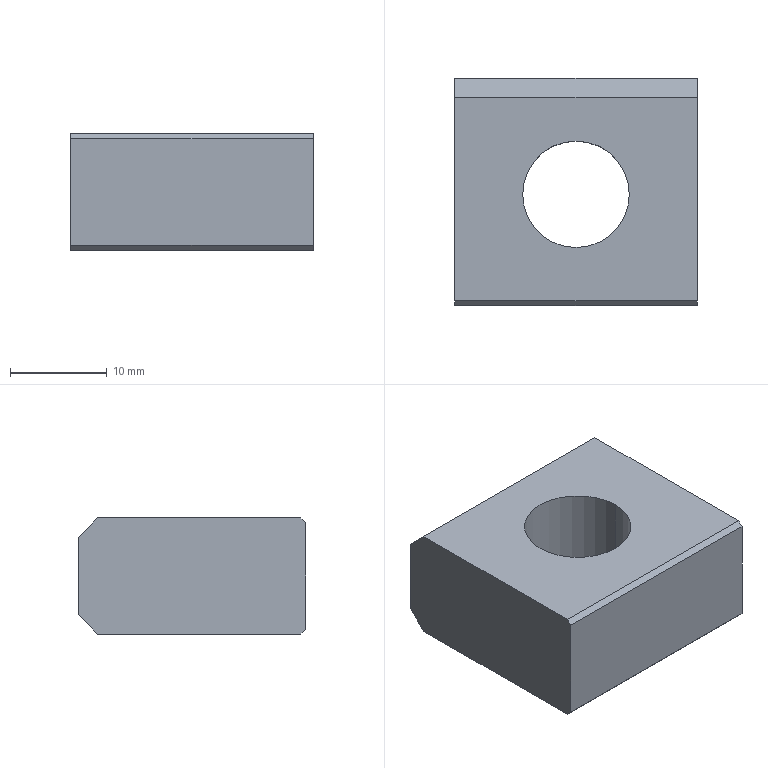Part | STEP file | 1 solid | 12 faces | box 25 x 23.5 x 12 mm | volume 5803 mm3 | plane 10 | cylinder 2 | commonest cylinder face diameters 11 x2
STEP:
#1=CARTESIAN_POINT('',(0.,0.,0.));
#2=DIRECTION('',(0.,0.,1.));
#3=DIRECTION('',(1.,0.,0.));
#4=AXIS2_PLACEMENT_3D('',#1,#2,#3);
#5=CARTESIAN_POINT('',(5.5,-0.25,-12.));
#6=VERTEX_POINT('',#5);
#7=CARTESIAN_POINT('',(5.5,-0.25,0.));
#8=VERTEX_POINT('',#7);
#9=CARTESIAN_POINT('',(5.5,-0.25,-12.));
#10=DIRECTION('',(0.,0.,1.));
#11=VECTOR('',#10,1.);
#12=LINE('',#9,#11);
#13=CARTESIAN_POINT('',(0.,-0.25,-12.));
#14=DIRECTION('',(0.,0.,1.));
#15=DIRECTION('',(1.,0.,0.));
#16=AXIS2_PLACEMENT_3D('',#13,#14,#15);
#17=CYLINDRICAL_SURFACE('',#16,5.5);
#18=CARTESIAN_POINT('',(6.283,0.));
#19=DIRECTION('',(0.,1.));
#20=VECTOR('',#19,1.);
#21=LINE('',#18,#20);
#22=(GEOMETRIC_REPRESENTATION_CONTEXT(2)PARAMETRIC_REPRESENTATION_CONTEXT()REPRESENTATION_CONTEXT('',''));
#23=DEFINITIONAL_REPRESENTATION('',(#21),#22);
#24=PCURVE('',#17,#23);
#25=CARTESIAN_POINT('',(0.,-0.25,-12.));
#26=DIRECTION('',(0.,0.,1.));
#27=DIRECTION('',(1.,0.,0.));
#28=AXIS2_PLACEMENT_3D('',#25,#26,#27);
#29=CYLINDRICAL_SURFACE('',#28,5.5);
#30=CARTESIAN_POINT('',(0.,0.));
#31=DIRECTION('',(0.,1.));
#32=VECTOR('',#31,1.);
#33=LINE('',#30,#32);
#34=(GEOMETRIC_REPRESENTATION_CONTEXT(2)PARAMETRIC_REPRESENTATION_CONTEXT()REPRESENTATION_CONTEXT('',''));
#35=DEFINITIONAL_REPRESENTATION('',(#33),#34);
#36=PCURVE('',#29,#35);
#37=SURFACE_CURVE('',#12,(#24,#36),.PCURVE_S1.);
#38=EDGE_CURVE('',#6,#8,#37,.T.);
#39=ORIENTED_EDGE('',*,*,#38,.T.);
#40=CARTESIAN_POINT('',(-5.5,-0.25,0.));
#41=VERTEX_POINT('',#40);
#42=CARTESIAN_POINT('',(0.,-0.25,0.));
#43=DIRECTION('',(0.,0.,1.));
#44=DIRECTION('',(1.,0.,0.));
#45=AXIS2_PLACEMENT_3D('',#42,#43,#44);
#46=CIRCLE('',#45,5.5);
#47=CARTESIAN_POINT('',(0.,12.));
#48=DIRECTION('',(1.,0.));
#49=VECTOR('',#48,1.);
#50=LINE('',#47,#49);
#51=(GEOMETRIC_REPRESENTATION_CONTEXT(2)PARAMETRIC_REPRESENTATION_CONTEXT()REPRESENTATION_CONTEXT('',''));
#52=DEFINITIONAL_REPRESENTATION('',(#50),#51);
#53=PCURVE('',#17,#52);
#54=CARTESIAN_POINT('',(-12.5,-11.75,0.));
#55=DIRECTION('',(0.,0.,-1.));
#56=DIRECTION('',(-1.,0.,0.));
#57=AXIS2_PLACEMENT_3D('',#54,#55,#56);
#58=PLANE('',#57);
#59=CARTESIAN_POINT('',(-18.,11.5));
#60=CARTESIAN_POINT('',(-18.,21.026));
#61=CARTESIAN_POINT('',(-9.75,16.263));
#62=CARTESIAN_POINT('',(-1.5,11.5));
#63=CARTESIAN_POINT('',(-9.75,6.737));
#64=CARTESIAN_POINT('',(-18.,1.974));
#65=CARTESIAN_POINT('',(-18.,11.5));
#66=(BOUNDED_CURVE()B_SPLINE_CURVE(2,(#59,#60,#61,#62,#63,#64,#65),.UNSPECIFIED.,.T.,.F.)B_SPLINE_CURVE_WITH_KNOTS((1,2,2,2,2,1),(-2.094,0.,2.094,4.189,6.283,8.378),.UNSPECIFIED.)CURVE()GEOMETRIC_REPRESENTATION_ITEM()RATIONAL_B_SPLINE_CURVE((1.,0.5,1.,0.5,1.,0.5,1.))REPRESENTATION_ITEM(''));
#67=(GEOMETRIC_REPRESENTATION_CONTEXT(2)PARAMETRIC_REPRESENTATION_CONTEXT()REPRESENTATION_CONTEXT('',''));
#68=DEFINITIONAL_REPRESENTATION('',(#66),#67);
#69=PCURVE('',#58,#68);
#70=SURFACE_CURVE('',#46,(#53,#69),.PCURVE_S1.);
#71=EDGE_CURVE('',#41,#8,#70,.T.);
#72=ORIENTED_EDGE('',*,*,#71,.F.);
#73=CARTESIAN_POINT('',(-5.5,-0.25,-12.));
#74=VERTEX_POINT('',#73);
#75=CARTESIAN_POINT('',(-5.5,-0.25,-12.));
#76=DIRECTION('',(0.,0.,1.));
#77=VECTOR('',#76,1.);
#78=LINE('',#75,#77);
#79=CARTESIAN_POINT('',(3.142,0.));
#80=DIRECTION('',(0.,1.));
#81=VECTOR('',#80,1.);
#82=LINE('',#79,#81);
#83=(GEOMETRIC_REPRESENTATION_CONTEXT(2)PARAMETRIC_REPRESENTATION_CONTEXT()REPRESENTATION_CONTEXT('',''));
#84=DEFINITIONAL_REPRESENTATION('',(#82),#83);
#85=PCURVE('',#17,#84);
#86=CARTESIAN_POINT('',(3.142,0.));
#87=DIRECTION('',(0.,1.));
#88=VECTOR('',#87,1.);
#89=LINE('',#86,#88);
#90=(GEOMETRIC_REPRESENTATION_CONTEXT(2)PARAMETRIC_REPRESENTATION_CONTEXT()REPRESENTATION_CONTEXT('',''));
#91=DEFINITIONAL_REPRESENTATION('',(#89),#90);
#92=PCURVE('',#29,#91);
#93=SURFACE_CURVE('',#78,(#85,#92),.PCURVE_S1.);
#94=EDGE_CURVE('',#74,#41,#93,.T.);
#95=ORIENTED_EDGE('',*,*,#94,.F.);
#96=CARTESIAN_POINT('',(0.,-0.25,-12.));
#97=DIRECTION('',(0.,0.,1.));
#98=DIRECTION('',(1.,0.,0.));
#99=AXIS2_PLACEMENT_3D('',#96,#97,#98);
#100=CIRCLE('',#99,5.5);
#101=CARTESIAN_POINT('',(0.,0.));
#102=DIRECTION('',(1.,0.));
#103=VECTOR('',#102,1.);
#104=LINE('',#101,#103);
#105=(GEOMETRIC_REPRESENTATION_CONTEXT(2)PARAMETRIC_REPRESENTATION_CONTEXT()REPRESENTATION_CONTEXT('',''));
#106=DEFINITIONAL_REPRESENTATION('',(#104),#105);
#107=PCURVE('',#17,#106);
#108=CARTESIAN_POINT('',(-12.5,-11.75,-12.));
#109=DIRECTION('',(0.,0.,-1.));
#110=DIRECTION('',(-1.,0.,0.));
#111=AXIS2_PLACEMENT_3D('',#108,#109,#110);
#112=PLANE('',#111);
#113=CARTESIAN_POINT('',(-18.,11.5));
#114=CARTESIAN_POINT('',(-18.,21.026));
#115=CARTESIAN_POINT('',(-9.75,16.263));
#116=CARTESIAN_POINT('',(-1.5,11.5));
#117=CARTESIAN_POINT('',(-9.75,6.737));
#118=CARTESIAN_POINT('',(-18.,1.974));
#119=CARTESIAN_POINT('',(-18.,11.5));
#120=(BOUNDED_CURVE()B_SPLINE_CURVE(2,(#113,#114,#115,#116,#117,#118,#119),.UNSPECIFIED.,.T.,.F.)B_SPLINE_CURVE_WITH_KNOTS((1,2,2,2,2,1),(-2.094,0.,2.094,4.189,6.283,8.378),.UNSPECIFIED.)CURVE()GEOMETRIC_REPRESENTATION_ITEM()RATIONAL_B_SPLINE_CURVE((1.,0.5,1.,0.5,1.,0.5,1.))REPRESENTATION_ITEM(''));
#121=(GEOMETRIC_REPRESENTATION_CONTEXT(2)PARAMETRIC_REPRESENTATION_CONTEXT()REPRESENTATION_CONTEXT('',''));
#122=DEFINITIONAL_REPRESENTATION('',(#120),#121);
#123=PCURVE('',#112,#122);
#124=SURFACE_CURVE('',#100,(#107,#123),.PCURVE_S1.);
#125=EDGE_CURVE('',#74,#6,#124,.T.);
#126=ORIENTED_EDGE('',*,*,#125,.T.);
#127=EDGE_LOOP('',(#39,#72,#95,#126));
#128=FACE_BOUND('',#127,.F.);
#129=ADVANCED_FACE('',(#128),#17,.F.);
#130=CARTESIAN_POINT('',(-12.5,9.75,-12.));
#131=VERTEX_POINT('',#130);
#132=CARTESIAN_POINT('',(-12.5,-11.25,-12.));
#133=VERTEX_POINT('',#132);
#134=CARTESIAN_POINT('',(-12.5,11.75,-12.));
#135=DIRECTION('',(0.,-1.,0.));
#136=VECTOR('',#135,1.);
#137=LINE('',#134,#136);
#138=CARTESIAN_POINT('',(-12.5,11.75,-12.));
#139=DIRECTION('',(-1.,0.,0.));
#140=DIRECTION('',(0.,-1.,0.));
#141=AXIS2_PLACEMENT_3D('',#138,#139,#140);
#142=PLANE('',#141);
#143=CARTESIAN_POINT('',(0.,0.));
#144=DIRECTION('',(1.,0.));
#145=VECTOR('',#144,1.);
#146=LINE('',#143,#145);
#147=(GEOMETRIC_REPRESENTATION_CONTEXT(2)PARAMETRIC_REPRESENTATION_CONTEXT()REPRESENTATION_CONTEXT('',''));
#148=DEFINITIONAL_REPRESENTATION('',(#146),#147);
#149=PCURVE('',#142,#148);
#150=CARTESIAN_POINT('',(0.,23.5));
#151=DIRECTION('',(0.,-1.));
#152=VECTOR('',#151,1.);
#153=LINE('',#150,#152);
#154=(GEOMETRIC_REPRESENTATION_CONTEXT(2)PARAMETRIC_REPRESENTATION_CONTEXT()REPRESENTATION_CONTEXT('',''));
#155=DEFINITIONAL_REPRESENTATION('',(#153),#154);
#156=PCURVE('',#112,#155);
#157=SURFACE_CURVE('',#137,(#149,#156),.PCURVE_S1.);
#158=EDGE_CURVE('',#131,#133,#157,.T.);
#159=ORIENTED_EDGE('',*,*,#158,.T.);
#160=CARTESIAN_POINT('',(-12.5,-11.75,-11.5));
#161=VERTEX_POINT('',#160);
#162=CARTESIAN_POINT('',(-12.5,0.25,-23.5));
#163=DIRECTION('',(0.,-0.7071,0.7071));
#164=VECTOR('',#163,1.);
#165=LINE('',#162,#164);
#166=CARTESIAN_POINT('',(11.5,-11.5));
#167=DIRECTION('',(0.7071,0.7071));
#168=VECTOR('',#167,1.);
#169=LINE('',#166,#168);
#170=(GEOMETRIC_REPRESENTATION_CONTEXT(2)PARAMETRIC_REPRESENTATION_CONTEXT()REPRESENTATION_CONTEXT('',''));
#171=DEFINITIONAL_REPRESENTATION('',(#169),#170);
#172=PCURVE('',#142,#171);
#173=CARTESIAN_POINT('',(12.5,-11.75,-11.5));
#174=DIRECTION('',(0.,0.7071,0.7071));
#175=DIRECTION('',(0.,-0.7071,0.7071));
#176=AXIS2_PLACEMENT_3D('',#173,#174,#175);
#177=PLANE('',#176);
#178=CARTESIAN_POINT('',(-16.971,-25.));
#179=DIRECTION('',(1.,0.));
#180=VECTOR('',#179,1.);
#181=LINE('',#178,#180);
#182=(GEOMETRIC_REPRESENTATION_CONTEXT(2)PARAMETRIC_REPRESENTATION_CONTEXT()REPRESENTATION_CONTEXT('',''));
#183=DEFINITIONAL_REPRESENTATION('',(#181),#182);
#184=PCURVE('',#177,#183);
#185=SURFACE_CURVE('',#165,(#172,#184),.PCURVE_S1.);
#186=EDGE_CURVE('',#133,#161,#185,.T.);
#187=ORIENTED_EDGE('',*,*,#186,.T.);
#188=CARTESIAN_POINT('',(-12.5,-11.75,-0.5));
#189=VERTEX_POINT('',#188);
#190=CARTESIAN_POINT('',(-12.5,-11.75,-12.));
#191=DIRECTION('',(0.,0.,1.));
#192=VECTOR('',#191,1.);
#193=LINE('',#190,#192);
#194=CARTESIAN_POINT('',(23.5,0.));
#195=DIRECTION('',(0.,1.));
#196=VECTOR('',#195,1.);
#197=LINE('',#194,#196);
#198=(GEOMETRIC_REPRESENTATION_CONTEXT(2)PARAMETRIC_REPRESENTATION_CONTEXT()REPRESENTATION_CONTEXT('',''));
#199=DEFINITIONAL_REPRESENTATION('',(#197),#198);
#200=PCURVE('',#142,#199);
#201=CARTESIAN_POINT('',(12.5,-11.75,-12.));
#202=DIRECTION('',(0.,-1.,0.));
#203=DIRECTION('',(1.,0.,0.));
#204=AXIS2_PLACEMENT_3D('',#201,#202,#203);
#205=PLANE('',#204);
#206=CARTESIAN_POINT('',(-25.,0.));
#207=DIRECTION('',(0.,1.));
#208=VECTOR('',#207,1.);
#209=LINE('',#206,#208);
#210=(GEOMETRIC_REPRESENTATION_CONTEXT(2)PARAMETRIC_REPRESENTATION_CONTEXT()REPRESENTATION_CONTEXT('',''));
#211=DEFINITIONAL_REPRESENTATION('',(#209),#210);
#212=PCURVE('',#205,#211);
#213=SURFACE_CURVE('',#193,(#200,#212),.PCURVE_S1.);
#214=EDGE_CURVE('',#161,#189,#213,.T.);
#215=ORIENTED_EDGE('',*,*,#214,.T.);
#216=CARTESIAN_POINT('',(-12.5,-11.25,0.));
#217=VERTEX_POINT('',#216);
#218=CARTESIAN_POINT('',(-12.5,-5.75,5.5));
#219=DIRECTION('',(0.,0.7071,0.7071));
#220=VECTOR('',#219,1.);
#221=LINE('',#218,#220);
#222=CARTESIAN_POINT('',(17.5,17.5));
#223=DIRECTION('',(-0.7071,0.7071));
#224=VECTOR('',#223,1.);
#225=LINE('',#222,#224);
#226=(GEOMETRIC_REPRESENTATION_CONTEXT(2)PARAMETRIC_REPRESENTATION_CONTEXT()REPRESENTATION_CONTEXT('',''));
#227=DEFINITIONAL_REPRESENTATION('',(#225),#226);
#228=PCURVE('',#142,#227);
#229=CARTESIAN_POINT('',(-12.5,-11.25,0.));
#230=DIRECTION('',(0.,-0.7071,0.7071));
#231=DIRECTION('',(0.,-0.7071,-0.7071));
#232=AXIS2_PLACEMENT_3D('',#229,#230,#231);
#233=PLANE('',#232);
#234=CARTESIAN_POINT('',(-7.778,0.));
#235=DIRECTION('',(-1.,0.));
#236=VECTOR('',#235,1.);
#237=LINE('',#234,#236);
#238=(GEOMETRIC_REPRESENTATION_CONTEXT(2)PARAMETRIC_REPRESENTATION_CONTEXT()REPRESENTATION_CONTEXT('',''));
#239=DEFINITIONAL_REPRESENTATION('',(#237),#238);
#240=PCURVE('',#233,#239);
#241=SURFACE_CURVE('',#221,(#228,#240),.PCURVE_S1.);
#242=EDGE_CURVE('',#189,#217,#241,.T.);
#243=ORIENTED_EDGE('',*,*,#242,.T.);
#244=CARTESIAN_POINT('',(-12.5,9.75,0.));
#245=VERTEX_POINT('',#244);
#246=CARTESIAN_POINT('',(-12.5,11.75,0.));
#247=DIRECTION('',(0.,-1.,0.));
#248=VECTOR('',#247,1.);
#249=LINE('',#246,#248);
#250=CARTESIAN_POINT('',(0.,12.));
#251=DIRECTION('',(1.,0.));
#252=VECTOR('',#251,1.);
#253=LINE('',#250,#252);
#254=(GEOMETRIC_REPRESENTATION_CONTEXT(2)PARAMETRIC_REPRESENTATION_CONTEXT()REPRESENTATION_CONTEXT('',''));
#255=DEFINITIONAL_REPRESENTATION('',(#253),#254);
#256=PCURVE('',#142,#255);
#257=CARTESIAN_POINT('',(0.,23.5));
#258=DIRECTION('',(0.,-1.));
#259=VECTOR('',#258,1.);
#260=LINE('',#257,#259);
#261=(GEOMETRIC_REPRESENTATION_CONTEXT(2)PARAMETRIC_REPRESENTATION_CONTEXT()REPRESENTATION_CONTEXT('',''));
#262=DEFINITIONAL_REPRESENTATION('',(#260),#261);
#263=PCURVE('',#58,#262);
#264=SURFACE_CURVE('',#249,(#256,#263),.PCURVE_S1.);
#265=EDGE_CURVE('',#245,#217,#264,.T.);
#266=ORIENTED_EDGE('',*,*,#265,.F.);
#267=CARTESIAN_POINT('',(-12.5,11.75,-2.));
#268=VERTEX_POINT('',#267);
#269=CARTESIAN_POINT('',(-12.5,16.75,-7.));
#270=DIRECTION('',(0.,0.7071,-0.7071));
#271=VECTOR('',#270,1.);
#272=LINE('',#269,#271);
#273=CARTESIAN_POINT('',(-5.,5.));
#274=DIRECTION('',(-0.7071,-0.7071));
#275=VECTOR('',#274,1.);
#276=LINE('',#273,#275);
#277=(GEOMETRIC_REPRESENTATION_CONTEXT(2)PARAMETRIC_REPRESENTATION_CONTEXT()REPRESENTATION_CONTEXT('',''));
#278=DEFINITIONAL_REPRESENTATION('',(#276),#277);
#279=PCURVE('',#142,#278);
#280=CARTESIAN_POINT('',(-12.5,9.75,0.));
#281=DIRECTION('',(0.,0.7071,0.7071));
#282=DIRECTION('',(0.,-0.7071,0.7071));
#283=AXIS2_PLACEMENT_3D('',#280,#281,#282);
#284=PLANE('',#283);
#285=CARTESIAN_POINT('',(-9.899,0.));
#286=DIRECTION('',(-1.,0.));
#287=VECTOR('',#286,1.);
#288=LINE('',#285,#287);
#289=(GEOMETRIC_REPRESENTATION_CONTEXT(2)PARAMETRIC_REPRESENTATION_CONTEXT()REPRESENTATION_CONTEXT('',''));
#290=DEFINITIONAL_REPRESENTATION('',(#288),#289);
#291=PCURVE('',#284,#290);
#292=SURFACE_CURVE('',#272,(#279,#291),.PCURVE_S1.);
#293=EDGE_CURVE('',#245,#268,#292,.T.);
#294=ORIENTED_EDGE('',*,*,#293,.T.);
#295=CARTESIAN_POINT('',(-12.5,11.75,-10.));
#296=VERTEX_POINT('',#295);
#297=CARTESIAN_POINT('',(-12.5,11.75,-12.));
#298=DIRECTION('',(0.,0.,1.));
#299=VECTOR('',#298,1.);
#300=LINE('',#297,#299);
#301=CARTESIAN_POINT('',(0.,0.));
#302=DIRECTION('',(0.,1.));
#303=VECTOR('',#302,1.);
#304=LINE('',#301,#303);
#305=(GEOMETRIC_REPRESENTATION_CONTEXT(2)PARAMETRIC_REPRESENTATION_CONTEXT()REPRESENTATION_CONTEXT('',''));
#306=DEFINITIONAL_REPRESENTATION('',(#304),#305);
#307=PCURVE('',#142,#306);
#308=CARTESIAN_POINT('',(12.5,11.75,-12.));
#309=DIRECTION('',(0.,1.,0.));
#310=DIRECTION('',(-1.,0.,0.));
#311=AXIS2_PLACEMENT_3D('',#308,#309,#310);
#312=PLANE('',#311);
#313=CARTESIAN_POINT('',(25.,0.));
#314=DIRECTION('',(0.,1.));
#315=VECTOR('',#314,1.);
#316=LINE('',#313,#315);
#317=(GEOMETRIC_REPRESENTATION_CONTEXT(2)PARAMETRIC_REPRESENTATION_CONTEXT()REPRESENTATION_CONTEXT('',''));
#318=DEFINITIONAL_REPRESENTATION('',(#316),#317);
#319=PCURVE('',#312,#318);
#320=SURFACE_CURVE('',#300,(#307,#319),.PCURVE_S1.);
#321=EDGE_CURVE('',#296,#268,#320,.T.);
#322=ORIENTED_EDGE('',*,*,#321,.F.);
#323=CARTESIAN_POINT('',(-12.5,10.75,-11.));
#324=DIRECTION('',(0.,-0.7071,-0.7071));
#325=VECTOR('',#324,1.);
#326=LINE('',#323,#325);
#327=CARTESIAN_POINT('',(1.,1.));
#328=DIRECTION('',(0.7071,-0.7071));
#329=VECTOR('',#328,1.);
#330=LINE('',#327,#329);
#331=(GEOMETRIC_REPRESENTATION_CONTEXT(2)PARAMETRIC_REPRESENTATION_CONTEXT()REPRESENTATION_CONTEXT('',''));
#332=DEFINITIONAL_REPRESENTATION('',(#330),#331);
#333=PCURVE('',#142,#332);
#334=CARTESIAN_POINT('',(12.5,11.75,-10.));
#335=DIRECTION('',(0.,-0.7071,0.7071));
#336=DIRECTION('',(0.,-0.7071,-0.7071));
#337=AXIS2_PLACEMENT_3D('',#334,#335,#336);
#338=PLANE('',#337);
#339=CARTESIAN_POINT('',(1.414,-25.));
#340=DIRECTION('',(1.,0.));
#341=VECTOR('',#340,1.);
#342=LINE('',#339,#341);
#343=(GEOMETRIC_REPRESENTATION_CONTEXT(2)PARAMETRIC_REPRESENTATION_CONTEXT()REPRESENTATION_CONTEXT('',''));
#344=DEFINITIONAL_REPRESENTATION('',(#342),#343);
#345=PCURVE('',#338,#344);
#346=SURFACE_CURVE('',#326,(#333,#345),.PCURVE_S1.);
#347=EDGE_CURVE('',#296,#131,#346,.T.);
#348=ORIENTED_EDGE('',*,*,#347,.T.);
#349=EDGE_LOOP('',(#159,#187,#215,#243,#266,#294,#322,#348));
#350=FACE_BOUND('',#349,.T.);
#351=ADVANCED_FACE('',(#350),#142,.T.);
#352=CARTESIAN_POINT('',(12.5,11.75,-10.));
#353=VERTEX_POINT('',#352);
#354=CARTESIAN_POINT('',(12.5,11.75,-2.));
#355=VERTEX_POINT('',#354);
#356=CARTESIAN_POINT('',(12.5,11.75,-12.));
#357=DIRECTION('',(0.,0.,1.));
#358=VECTOR('',#357,1.);
#359=LINE('',#356,#358);
#360=CARTESIAN_POINT('',(0.,0.));
#361=DIRECTION('',(0.,1.));
#362=VECTOR('',#361,1.);
#363=LINE('',#360,#362);
#364=(GEOMETRIC_REPRESENTATION_CONTEXT(2)PARAMETRIC_REPRESENTATION_CONTEXT()REPRESENTATION_CONTEXT('',''));
#365=DEFINITIONAL_REPRESENTATION('',(#363),#364);
#366=PCURVE('',#312,#365);
#367=CARTESIAN_POINT('',(12.5,11.75,-12.));
#368=DIRECTION('',(1.,0.,0.));
#369=DIRECTION('',(0.,1.,0.));
#370=AXIS2_PLACEMENT_3D('',#367,#368,#369);
#371=PLANE('',#370);
#372=CARTESIAN_POINT('',(0.,0.));
#373=DIRECTION('',(0.,1.));
#374=VECTOR('',#373,1.);
#375=LINE('',#372,#374);
#376=(GEOMETRIC_REPRESENTATION_CONTEXT(2)PARAMETRIC_REPRESENTATION_CONTEXT()REPRESENTATION_CONTEXT('',''));
#377=DEFINITIONAL_REPRESENTATION('',(#375),#376);
#378=PCURVE('',#371,#377);
#379=SURFACE_CURVE('',#359,(#366,#378),.PCURVE_S1.);
#380=EDGE_CURVE('',#353,#355,#379,.T.);
#381=ORIENTED_EDGE('',*,*,#380,.F.);
#382=CARTESIAN_POINT('',(12.5,11.75,-10.));
#383=DIRECTION('',(-1.,0.,0.));
#384=VECTOR('',#383,1.);
#385=LINE('',#382,#384);
#386=CARTESIAN_POINT('',(0.,2.));
#387=DIRECTION('',(1.,0.));
#388=VECTOR('',#387,1.);
#389=LINE('',#386,#388);
#390=(GEOMETRIC_REPRESENTATION_CONTEXT(2)PARAMETRIC_REPRESENTATION_CONTEXT()REPRESENTATION_CONTEXT('',''));
#391=DEFINITIONAL_REPRESENTATION('',(#389),#390);
#392=PCURVE('',#312,#391);
#393=CARTESIAN_POINT('',(0.,0.));
#394=DIRECTION('',(0.,-1.));
#395=VECTOR('',#394,1.);
#396=LINE('',#393,#395);
#397=(GEOMETRIC_REPRESENTATION_CONTEXT(2)PARAMETRIC_REPRESENTATION_CONTEXT()REPRESENTATION_CONTEXT('',''));
#398=DEFINITIONAL_REPRESENTATION('',(#396),#397);
#399=PCURVE('',#338,#398);
#400=SURFACE_CURVE('',#385,(#392,#399),.PCURVE_S1.);
#401=EDGE_CURVE('',#353,#296,#400,.T.);
#402=ORIENTED_EDGE('',*,*,#401,.T.);
#403=ORIENTED_EDGE('',*,*,#321,.T.);
#404=CARTESIAN_POINT('',(12.5,11.75,-2.));
#405=DIRECTION('',(1.,0.,0.));
#406=VECTOR('',#405,1.);
#407=LINE('',#404,#406);
#408=CARTESIAN_POINT('',(0.,10.));
#409=DIRECTION('',(-1.,0.));
#410=VECTOR('',#409,1.);
#411=LINE('',#408,#410);
#412=(GEOMETRIC_REPRESENTATION_CONTEXT(2)PARAMETRIC_REPRESENTATION_CONTEXT()REPRESENTATION_CONTEXT('',''));
#413=DEFINITIONAL_REPRESENTATION('',(#411),#412);
#414=PCURVE('',#312,#413);
#415=CARTESIAN_POINT('',(-2.828,25.));
#416=DIRECTION('',(0.,1.));
#417=VECTOR('',#416,1.);
#418=LINE('',#415,#417);
#419=(GEOMETRIC_REPRESENTATION_CONTEXT(2)PARAMETRIC_REPRESENTATION_CONTEXT()REPRESENTATION_CONTEXT('',''));
#420=DEFINITIONAL_REPRESENTATION('',(#418),#419);
#421=PCURVE('',#284,#420);
#422=SURFACE_CURVE('',#407,(#414,#421),.PCURVE_S1.);
#423=EDGE_CURVE('',#268,#355,#422,.T.);
#424=ORIENTED_EDGE('',*,*,#423,.T.);
#425=EDGE_LOOP('',(#381,#402,#403,#424));
#426=FACE_BOUND('',#425,.T.);
#427=ADVANCED_FACE('',(#426),#312,.T.);
#428=CARTESIAN_POINT('',(12.5,-11.75,-11.5));
#429=VERTEX_POINT('',#428);
#430=CARTESIAN_POINT('',(12.5,-11.75,-0.5));
#431=VERTEX_POINT('',#430);
#432=CARTESIAN_POINT('',(12.5,-11.75,-12.));
#433=DIRECTION('',(0.,0.,1.));
#434=VECTOR('',#433,1.);
#435=LINE('',#432,#434);
#436=CARTESIAN_POINT('',(-23.5,0.));
#437=DIRECTION('',(0.,1.));
#438=VECTOR('',#437,1.);
#439=LINE('',#436,#438);
#440=(GEOMETRIC_REPRESENTATION_CONTEXT(2)PARAMETRIC_REPRESENTATION_CONTEXT()REPRESENTATION_CONTEXT('',''));
#441=DEFINITIONAL_REPRESENTATION('',(#439),#440);
#442=PCURVE('',#371,#441);
#443=CARTESIAN_POINT('',(0.,0.));
#444=DIRECTION('',(0.,1.));
#445=VECTOR('',#444,1.);
#446=LINE('',#443,#445);
#447=(GEOMETRIC_REPRESENTATION_CONTEXT(2)PARAMETRIC_REPRESENTATION_CONTEXT()REPRESENTATION_CONTEXT('',''));
#448=DEFINITIONAL_REPRESENTATION('',(#446),#447);
#449=PCURVE('',#205,#448);
#450=SURFACE_CURVE('',#435,(#442,#449),.PCURVE_S1.);
#451=EDGE_CURVE('',#429,#431,#450,.T.);
#452=ORIENTED_EDGE('',*,*,#451,.F.);
#453=CARTESIAN_POINT('',(12.5,-11.25,-12.));
#454=VERTEX_POINT('',#453);
#455=CARTESIAN_POINT('',(12.5,0.25,-23.5));
#456=DIRECTION('',(0.,0.7071,-0.7071));
#457=VECTOR('',#456,1.);
#458=LINE('',#455,#457);
#459=CARTESIAN_POINT('',(-11.5,-11.5));
#460=DIRECTION('',(0.7071,-0.7071));
#461=VECTOR('',#460,1.);
#462=LINE('',#459,#461);
#463=(GEOMETRIC_REPRESENTATION_CONTEXT(2)PARAMETRIC_REPRESENTATION_CONTEXT()REPRESENTATION_CONTEXT('',''));
#464=DEFINITIONAL_REPRESENTATION('',(#462),#463);
#465=PCURVE('',#371,#464);
#466=CARTESIAN_POINT('',(-16.971,0.));
#467=DIRECTION('',(-1.,0.));
#468=VECTOR('',#467,1.);
#469=LINE('',#466,#468);
#470=(GEOMETRIC_REPRESENTATION_CONTEXT(2)PARAMETRIC_REPRESENTATION_CONTEXT()REPRESENTATION_CONTEXT('',''));
#471=DEFINITIONAL_REPRESENTATION('',(#469),#470);
#472=PCURVE('',#177,#471);
#473=SURFACE_CURVE('',#458,(#465,#472),.PCURVE_S1.);
#474=EDGE_CURVE('',#429,#454,#473,.T.);
#475=ORIENTED_EDGE('',*,*,#474,.T.);
#476=CARTESIAN_POINT('',(12.5,9.75,-12.));
#477=VERTEX_POINT('',#476);
#478=CARTESIAN_POINT('',(12.5,11.75,-12.));
#479=DIRECTION('',(0.,1.,0.));
#480=VECTOR('',#479,1.);
#481=LINE('',#478,#480);
#482=CARTESIAN_POINT('',(0.,0.));
#483=DIRECTION('',(1.,0.));
#484=VECTOR('',#483,1.);
#485=LINE('',#482,#484);
#486=(GEOMETRIC_REPRESENTATION_CONTEXT(2)PARAMETRIC_REPRESENTATION_CONTEXT()REPRESENTATION_CONTEXT('',''));
#487=DEFINITIONAL_REPRESENTATION('',(#485),#486);
#488=PCURVE('',#371,#487);
#489=CARTESIAN_POINT('',(-25.,23.5));
#490=DIRECTION('',(0.,1.));
#491=VECTOR('',#490,1.);
#492=LINE('',#489,#491);
#493=(GEOMETRIC_REPRESENTATION_CONTEXT(2)PARAMETRIC_REPRESENTATION_CONTEXT()REPRESENTATION_CONTEXT('',''));
#494=DEFINITIONAL_REPRESENTATION('',(#492),#493);
#495=PCURVE('',#112,#494);
#496=SURFACE_CURVE('',#481,(#488,#495),.PCURVE_S1.);
#497=EDGE_CURVE('',#454,#477,#496,.T.);
#498=ORIENTED_EDGE('',*,*,#497,.T.);
#499=CARTESIAN_POINT('',(12.5,10.75,-11.));
#500=DIRECTION('',(0.,0.7071,0.7071));
#501=VECTOR('',#500,1.);
#502=LINE('',#499,#501);
#503=CARTESIAN_POINT('',(-1.,1.));
#504=DIRECTION('',(0.7071,0.7071));
#505=VECTOR('',#504,1.);
#506=LINE('',#503,#505);
#507=(GEOMETRIC_REPRESENTATION_CONTEXT(2)PARAMETRIC_REPRESENTATION_CONTEXT()REPRESENTATION_CONTEXT('',''));
#508=DEFINITIONAL_REPRESENTATION('',(#506),#507);
#509=PCURVE('',#371,#508);
#510=CARTESIAN_POINT('',(1.414,0.));
#511=DIRECTION('',(-1.,0.));
#512=VECTOR('',#511,1.);
#513=LINE('',#510,#512);
#514=(GEOMETRIC_REPRESENTATION_CONTEXT(2)PARAMETRIC_REPRESENTATION_CONTEXT()REPRESENTATION_CONTEXT('',''));
#515=DEFINITIONAL_REPRESENTATION('',(#513),#514);
#516=PCURVE('',#338,#515);
#517=SURFACE_CURVE('',#502,(#509,#516),.PCURVE_S1.);
#518=EDGE_CURVE('',#477,#353,#517,.T.);
#519=ORIENTED_EDGE('',*,*,#518,.T.);
#520=ORIENTED_EDGE('',*,*,#380,.T.);
#521=CARTESIAN_POINT('',(12.5,9.75,0.));
#522=VERTEX_POINT('',#521);
#523=CARTESIAN_POINT('',(12.5,16.75,-7.));
#524=DIRECTION('',(0.,-0.7071,0.7071));
#525=VECTOR('',#524,1.);
#526=LINE('',#523,#525);
#527=CARTESIAN_POINT('',(5.,5.));
#528=DIRECTION('',(-0.7071,0.7071));
#529=VECTOR('',#528,1.);
#530=LINE('',#527,#529);
#531=(GEOMETRIC_REPRESENTATION_CONTEXT(2)PARAMETRIC_REPRESENTATION_CONTEXT()REPRESENTATION_CONTEXT('',''));
#532=DEFINITIONAL_REPRESENTATION('',(#530),#531);
#533=PCURVE('',#371,#532);
#534=CARTESIAN_POINT('',(-9.899,25.));
#535=DIRECTION('',(1.,0.));
#536=VECTOR('',#535,1.);
#537=LINE('',#534,#536);
#538=(GEOMETRIC_REPRESENTATION_CONTEXT(2)PARAMETRIC_REPRESENTATION_CONTEXT()REPRESENTATION_CONTEXT('',''));
#539=DEFINITIONAL_REPRESENTATION('',(#537),#538);
#540=PCURVE('',#284,#539);
#541=SURFACE_CURVE('',#526,(#533,#540),.PCURVE_S1.);
#542=EDGE_CURVE('',#355,#522,#541,.T.);
#543=ORIENTED_EDGE('',*,*,#542,.T.);
#544=CARTESIAN_POINT('',(12.5,-11.25,0.));
#545=VERTEX_POINT('',#544);
#546=CARTESIAN_POINT('',(12.5,11.75,0.));
#547=DIRECTION('',(0.,1.,0.));
#548=VECTOR('',#547,1.);
#549=LINE('',#546,#548);
#550=CARTESIAN_POINT('',(0.,12.));
#551=DIRECTION('',(1.,0.));
#552=VECTOR('',#551,1.);
#553=LINE('',#550,#552);
#554=(GEOMETRIC_REPRESENTATION_CONTEXT(2)PARAMETRIC_REPRESENTATION_CONTEXT()REPRESENTATION_CONTEXT('',''));
#555=DEFINITIONAL_REPRESENTATION('',(#553),#554);
#556=PCURVE('',#371,#555);
#557=CARTESIAN_POINT('',(-25.,23.5));
#558=DIRECTION('',(0.,1.));
#559=VECTOR('',#558,1.);
#560=LINE('',#557,#559);
#561=(GEOMETRIC_REPRESENTATION_CONTEXT(2)PARAMETRIC_REPRESENTATION_CONTEXT()REPRESENTATION_CONTEXT('',''));
#562=DEFINITIONAL_REPRESENTATION('',(#560),#561);
#563=PCURVE('',#58,#562);
#564=SURFACE_CURVE('',#549,(#556,#563),.PCURVE_S1.);
#565=EDGE_CURVE('',#545,#522,#564,.T.);
#566=ORIENTED_EDGE('',*,*,#565,.F.);
#567=CARTESIAN_POINT('',(12.5,-5.75,5.5));
#568=DIRECTION('',(0.,-0.7071,-0.7071));
#569=VECTOR('',#568,1.);
#570=LINE('',#567,#569);
#571=CARTESIAN_POINT('',(-17.5,17.5));
#572=DIRECTION('',(-0.7071,-0.7071));
#573=VECTOR('',#572,1.);
#574=LINE('',#571,#573);
#575=(GEOMETRIC_REPRESENTATION_CONTEXT(2)PARAMETRIC_REPRESENTATION_CONTEXT()REPRESENTATION_CONTEXT('',''));
#576=DEFINITIONAL_REPRESENTATION('',(#574),#575);
#577=PCURVE('',#371,#576);
#578=CARTESIAN_POINT('',(-7.778,25.));
#579=DIRECTION('',(1.,0.));
#580=VECTOR('',#579,1.);
#581=LINE('',#578,#580);
#582=(GEOMETRIC_REPRESENTATION_CONTEXT(2)PARAMETRIC_REPRESENTATION_CONTEXT()REPRESENTATION_CONTEXT('',''));
#583=DEFINITIONAL_REPRESENTATION('',(#581),#582);
#584=PCURVE('',#233,#583);
#585=SURFACE_CURVE('',#570,(#577,#584),.PCURVE_S1.);
#586=EDGE_CURVE('',#545,#431,#585,.T.);
#587=ORIENTED_EDGE('',*,*,#586,.T.);
#588=EDGE_LOOP('',(#452,#475,#498,#519,#520,#543,#566,#587));
#589=FACE_BOUND('',#588,.T.);
#590=ADVANCED_FACE('',(#589),#371,.T.);
#591=ORIENTED_EDGE('',*,*,#214,.F.);
#592=CARTESIAN_POINT('',(12.5,-11.75,-11.5));
#593=DIRECTION('',(1.,0.,0.));
#594=VECTOR('',#593,1.);
#595=LINE('',#592,#594);
#596=CARTESIAN_POINT('',(0.,0.5));
#597=DIRECTION('',(1.,0.));
#598=VECTOR('',#597,1.);
#599=LINE('',#596,#598);
#600=(GEOMETRIC_REPRESENTATION_CONTEXT(2)PARAMETRIC_REPRESENTATION_CONTEXT()REPRESENTATION_CONTEXT('',''));
#601=DEFINITIONAL_REPRESENTATION('',(#599),#600);
#602=PCURVE('',#205,#601);
#603=CARTESIAN_POINT('',(0.,0.));
#604=DIRECTION('',(0.,1.));
#605=VECTOR('',#604,1.);
#606=LINE('',#603,#605);
#607=(GEOMETRIC_REPRESENTATION_CONTEXT(2)PARAMETRIC_REPRESENTATION_CONTEXT()REPRESENTATION_CONTEXT('',''));
#608=DEFINITIONAL_REPRESENTATION('',(#606),#607);
#609=PCURVE('',#177,#608);
#610=SURFACE_CURVE('',#595,(#602,#609),.PCURVE_S1.);
#611=EDGE_CURVE('',#161,#429,#610,.T.);
#612=ORIENTED_EDGE('',*,*,#611,.T.);
#613=ORIENTED_EDGE('',*,*,#451,.T.);
#614=CARTESIAN_POINT('',(-12.5,-11.75,-0.5));
#615=DIRECTION('',(-1.,0.,0.));
#616=VECTOR('',#615,1.);
#617=LINE('',#614,#616);
#618=CARTESIAN_POINT('',(-25.,11.5));
#619=DIRECTION('',(-1.,0.));
#620=VECTOR('',#619,1.);
#621=LINE('',#618,#620);
#622=(GEOMETRIC_REPRESENTATION_CONTEXT(2)PARAMETRIC_REPRESENTATION_CONTEXT()REPRESENTATION_CONTEXT('',''));
#623=DEFINITIONAL_REPRESENTATION('',(#621),#622);
#624=PCURVE('',#205,#623);
#625=CARTESIAN_POINT('',(0.7071,0.));
#626=DIRECTION('',(0.,-1.));
#627=VECTOR('',#626,1.);
#628=LINE('',#625,#627);
#629=(GEOMETRIC_REPRESENTATION_CONTEXT(2)PARAMETRIC_REPRESENTATION_CONTEXT()REPRESENTATION_CONTEXT('',''));
#630=DEFINITIONAL_REPRESENTATION('',(#628),#629);
#631=PCURVE('',#233,#630);
#632=SURFACE_CURVE('',#617,(#624,#631),.PCURVE_S1.);
#633=EDGE_CURVE('',#431,#189,#632,.T.);
#634=ORIENTED_EDGE('',*,*,#633,.T.);
#635=EDGE_LOOP('',(#591,#612,#613,#634));
#636=FACE_BOUND('',#635,.T.);
#637=ADVANCED_FACE('',(#636),#205,.T.);
#638=CARTESIAN_POINT('',(0.,-0.25,-12.));
#639=DIRECTION('',(0.,0.,1.));
#640=DIRECTION('',(1.,0.,0.));
#641=AXIS2_PLACEMENT_3D('',#638,#639,#640);
#642=CIRCLE('',#641,5.5);
#643=CARTESIAN_POINT('',(-18.,11.5));
#644=CARTESIAN_POINT('',(-18.,21.026));
#645=CARTESIAN_POINT('',(-9.75,16.263));
#646=CARTESIAN_POINT('',(-1.5,11.5));
#647=CARTESIAN_POINT('',(-9.75,6.737));
#648=CARTESIAN_POINT('',(-18.,1.974));
#649=CARTESIAN_POINT('',(-18.,11.5));
#650=(BOUNDED_CURVE()B_SPLINE_CURVE(2,(#643,#644,#645,#646,#647,#648,#649),.UNSPECIFIED.,.T.,.F.)B_SPLINE_CURVE_WITH_KNOTS((1,2,2,2,2,1),(-2.094,0.,2.094,4.189,6.283,8.378),.UNSPECIFIED.)CURVE()GEOMETRIC_REPRESENTATION_ITEM()RATIONAL_B_SPLINE_CURVE((1.,0.5,1.,0.5,1.,0.5,1.))REPRESENTATION_ITEM(''));
#651=(GEOMETRIC_REPRESENTATION_CONTEXT(2)PARAMETRIC_REPRESENTATION_CONTEXT()REPRESENTATION_CONTEXT('',''));
#652=DEFINITIONAL_REPRESENTATION('',(#650),#651);
#653=PCURVE('',#112,#652);
#654=CARTESIAN_POINT('',(0.,0.));
#655=DIRECTION('',(1.,0.));
#656=VECTOR('',#655,1.);
#657=LINE('',#654,#656);
#658=(GEOMETRIC_REPRESENTATION_CONTEXT(2)PARAMETRIC_REPRESENTATION_CONTEXT()REPRESENTATION_CONTEXT('',''));
#659=DEFINITIONAL_REPRESENTATION('',(#657),#658);
#660=PCURVE('',#29,#659);
#661=SURFACE_CURVE('',#642,(#653,#660),.PCURVE_S1.);
#662=EDGE_CURVE('',#6,#74,#661,.T.);
#663=ORIENTED_EDGE('',*,*,#662,.T.);
#664=ORIENTED_EDGE('',*,*,#125,.T.);
#665=EDGE_LOOP('',(#663,#664));
#666=FACE_BOUND('',#665,.T.);
#667=ORIENTED_EDGE('',*,*,#497,.F.);
#668=CARTESIAN_POINT('',(-12.5,-11.25,-12.));
#669=DIRECTION('',(-1.,0.,0.));
#670=VECTOR('',#669,1.);
#671=LINE('',#668,#670);
#672=CARTESIAN_POINT('',(0.,0.5));
#673=DIRECTION('',(1.,0.));
#674=VECTOR('',#673,1.);
#675=LINE('',#672,#674);
#676=(GEOMETRIC_REPRESENTATION_CONTEXT(2)PARAMETRIC_REPRESENTATION_CONTEXT()REPRESENTATION_CONTEXT('',''));
#677=DEFINITIONAL_REPRESENTATION('',(#675),#676);
#678=PCURVE('',#112,#677);
#679=CARTESIAN_POINT('',(-0.7071,-25.));
#680=DIRECTION('',(0.,-1.));
#681=VECTOR('',#680,1.);
#682=LINE('',#679,#681);
#683=(GEOMETRIC_REPRESENTATION_CONTEXT(2)PARAMETRIC_REPRESENTATION_CONTEXT()REPRESENTATION_CONTEXT('',''));
#684=DEFINITIONAL_REPRESENTATION('',(#682),#683);
#685=PCURVE('',#177,#684);
#686=SURFACE_CURVE('',#671,(#678,#685),.PCURVE_S1.);
#687=EDGE_CURVE('',#454,#133,#686,.T.);
#688=ORIENTED_EDGE('',*,*,#687,.T.);
#689=ORIENTED_EDGE('',*,*,#158,.F.);
#690=CARTESIAN_POINT('',(-12.5,9.75,-12.));
#691=DIRECTION('',(1.,0.,0.));
#692=VECTOR('',#691,1.);
#693=LINE('',#690,#692);
#694=CARTESIAN_POINT('',(0.,21.5));
#695=DIRECTION('',(-1.,0.));
#696=VECTOR('',#695,1.);
#697=LINE('',#694,#696);
#698=(GEOMETRIC_REPRESENTATION_CONTEXT(2)PARAMETRIC_REPRESENTATION_CONTEXT()REPRESENTATION_CONTEXT('',''));
#699=DEFINITIONAL_REPRESENTATION('',(#697),#698);
#700=PCURVE('',#112,#699);
#701=CARTESIAN_POINT('',(2.828,-25.));
#702=DIRECTION('',(0.,1.));
#703=VECTOR('',#702,1.);
#704=LINE('',#701,#703);
#705=(GEOMETRIC_REPRESENTATION_CONTEXT(2)PARAMETRIC_REPRESENTATION_CONTEXT()REPRESENTATION_CONTEXT('',''));
#706=DEFINITIONAL_REPRESENTATION('',(#704),#705);
#707=PCURVE('',#338,#706);
#708=SURFACE_CURVE('',#693,(#700,#707),.PCURVE_S1.);
#709=EDGE_CURVE('',#131,#477,#708,.T.);
#710=ORIENTED_EDGE('',*,*,#709,.T.);
#711=EDGE_LOOP('',(#667,#688,#689,#710));
#712=FACE_BOUND('',#711,.T.);
#713=ADVANCED_FACE('',(#666,#712),#112,.T.);
#714=CARTESIAN_POINT('',(0.,-0.25,0.));
#715=DIRECTION('',(0.,0.,1.));
#716=DIRECTION('',(1.,0.,0.));
#717=AXIS2_PLACEMENT_3D('',#714,#715,#716);
#718=CIRCLE('',#717,5.5);
#719=CARTESIAN_POINT('',(-18.,11.5));
#720=CARTESIAN_POINT('',(-18.,21.026));
#721=CARTESIAN_POINT('',(-9.75,16.263));
#722=CARTESIAN_POINT('',(-1.5,11.5));
#723=CARTESIAN_POINT('',(-9.75,6.737));
#724=CARTESIAN_POINT('',(-18.,1.974));
#725=CARTESIAN_POINT('',(-18.,11.5));
#726=(BOUNDED_CURVE()B_SPLINE_CURVE(2,(#719,#720,#721,#722,#723,#724,#725),.UNSPECIFIED.,.T.,.F.)B_SPLINE_CURVE_WITH_KNOTS((1,2,2,2,2,1),(-2.094,0.,2.094,4.189,6.283,8.378),.UNSPECIFIED.)CURVE()GEOMETRIC_REPRESENTATION_ITEM()RATIONAL_B_SPLINE_CURVE((1.,0.5,1.,0.5,1.,0.5,1.))REPRESENTATION_ITEM(''));
#727=(GEOMETRIC_REPRESENTATION_CONTEXT(2)PARAMETRIC_REPRESENTATION_CONTEXT()REPRESENTATION_CONTEXT('',''));
#728=DEFINITIONAL_REPRESENTATION('',(#726),#727);
#729=PCURVE('',#58,#728);
#730=CARTESIAN_POINT('',(0.,12.));
#731=DIRECTION('',(1.,0.));
#732=VECTOR('',#731,1.);
#733=LINE('',#730,#732);
#734=(GEOMETRIC_REPRESENTATION_CONTEXT(2)PARAMETRIC_REPRESENTATION_CONTEXT()REPRESENTATION_CONTEXT('',''));
#735=DEFINITIONAL_REPRESENTATION('',(#733),#734);
#736=PCURVE('',#29,#735);
#737=SURFACE_CURVE('',#718,(#729,#736),.PCURVE_S1.);
#738=EDGE_CURVE('',#8,#41,#737,.T.);
#739=ORIENTED_EDGE('',*,*,#738,.F.);
#740=ORIENTED_EDGE('',*,*,#71,.F.);
#741=EDGE_LOOP('',(#739,#740));
#742=FACE_BOUND('',#741,.T.);
#743=ORIENTED_EDGE('',*,*,#265,.T.);
#744=CARTESIAN_POINT('',(12.5,-11.25,0.));
#745=DIRECTION('',(1.,0.,0.));
#746=VECTOR('',#745,1.);
#747=LINE('',#744,#746);
#748=CARTESIAN_POINT('',(-25.,0.5));
#749=DIRECTION('',(-1.,0.));
#750=VECTOR('',#749,1.);
#751=LINE('',#748,#750);
#752=(GEOMETRIC_REPRESENTATION_CONTEXT(2)PARAMETRIC_REPRESENTATION_CONTEXT()REPRESENTATION_CONTEXT('',''));
#753=DEFINITIONAL_REPRESENTATION('',(#751),#752);
#754=PCURVE('',#58,#753);
#755=CARTESIAN_POINT('',(0.,25.));
#756=DIRECTION('',(0.,1.));
#757=VECTOR('',#756,1.);
#758=LINE('',#755,#757);
#759=(GEOMETRIC_REPRESENTATION_CONTEXT(2)PARAMETRIC_REPRESENTATION_CONTEXT()REPRESENTATION_CONTEXT('',''));
#760=DEFINITIONAL_REPRESENTATION('',(#758),#759);
#761=PCURVE('',#233,#760);
#762=SURFACE_CURVE('',#747,(#754,#761),.PCURVE_S1.);
#763=EDGE_CURVE('',#217,#545,#762,.T.);
#764=ORIENTED_EDGE('',*,*,#763,.T.);
#765=ORIENTED_EDGE('',*,*,#565,.T.);
#766=CARTESIAN_POINT('',(-12.5,9.75,0.));
#767=DIRECTION('',(-1.,0.,0.));
#768=VECTOR('',#767,1.);
#769=LINE('',#766,#768);
#770=CARTESIAN_POINT('',(0.,21.5));
#771=DIRECTION('',(1.,0.));
#772=VECTOR('',#771,1.);
#773=LINE('',#770,#772);
#774=(GEOMETRIC_REPRESENTATION_CONTEXT(2)PARAMETRIC_REPRESENTATION_CONTEXT()REPRESENTATION_CONTEXT('',''));
#775=DEFINITIONAL_REPRESENTATION('',(#773),#774);
#776=PCURVE('',#58,#775);
#777=CARTESIAN_POINT('',(0.,0.));
#778=DIRECTION('',(0.,-1.));
#779=VECTOR('',#778,1.);
#780=LINE('',#777,#779);
#781=(GEOMETRIC_REPRESENTATION_CONTEXT(2)PARAMETRIC_REPRESENTATION_CONTEXT()REPRESENTATION_CONTEXT('',''));
#782=DEFINITIONAL_REPRESENTATION('',(#780),#781);
#783=PCURVE('',#284,#782);
#784=SURFACE_CURVE('',#769,(#776,#783),.PCURVE_S1.);
#785=EDGE_CURVE('',#522,#245,#784,.T.);
#786=ORIENTED_EDGE('',*,*,#785,.T.);
#787=EDGE_LOOP('',(#743,#764,#765,#786));
#788=FACE_BOUND('',#787,.T.);
#789=ADVANCED_FACE('',(#742,#788),#58,.F.);
#790=ORIENTED_EDGE('',*,*,#738,.F.);
#791=ORIENTED_EDGE('',*,*,#38,.F.);
#792=ORIENTED_EDGE('',*,*,#662,.T.);
#793=ORIENTED_EDGE('',*,*,#94,.T.);
#794=EDGE_LOOP('',(#790,#791,#792,#793));
#795=FACE_BOUND('',#794,.F.);
#796=ADVANCED_FACE('',(#795),#29,.F.);
#797=ORIENTED_EDGE('',*,*,#518,.F.);
#798=ORIENTED_EDGE('',*,*,#709,.F.);
#799=ORIENTED_EDGE('',*,*,#347,.F.);
#800=ORIENTED_EDGE('',*,*,#401,.F.);
#801=EDGE_LOOP('',(#797,#798,#799,#800));
#802=FACE_BOUND('',#801,.T.);
#803=ADVANCED_FACE('',(#802),#338,.F.);
#804=ORIENTED_EDGE('',*,*,#542,.F.);
#805=ORIENTED_EDGE('',*,*,#423,.F.);
#806=ORIENTED_EDGE('',*,*,#293,.F.);
#807=ORIENTED_EDGE('',*,*,#785,.F.);
#808=EDGE_LOOP('',(#804,#805,#806,#807));
#809=FACE_BOUND('',#808,.T.);
#810=ADVANCED_FACE('',(#809),#284,.T.);
#811=ORIENTED_EDGE('',*,*,#186,.F.);
#812=ORIENTED_EDGE('',*,*,#687,.F.);
#813=ORIENTED_EDGE('',*,*,#474,.F.);
#814=ORIENTED_EDGE('',*,*,#611,.F.);
#815=EDGE_LOOP('',(#811,#812,#813,#814));
#816=FACE_BOUND('',#815,.T.);
#817=ADVANCED_FACE('',(#816),#177,.F.);
#818=ORIENTED_EDGE('',*,*,#242,.F.);
#819=ORIENTED_EDGE('',*,*,#633,.F.);
#820=ORIENTED_EDGE('',*,*,#586,.F.);
#821=ORIENTED_EDGE('',*,*,#763,.F.);
#822=EDGE_LOOP('',(#818,#819,#820,#821));
#823=FACE_BOUND('',#822,.T.);
#824=ADVANCED_FACE('',(#823),#233,.T.);
#825=CLOSED_SHELL('',(#129,#351,#427,#590,#637,#713,#789,#796,#803,#810,#817,#824));
#826=MANIFOLD_SOLID_BREP('',#825);
#827=(LENGTH_UNIT()NAMED_UNIT(*)SI_UNIT(.MILLI.,.METRE.));
#828=UNCERTAINTY_MEASURE_WITH_UNIT(LENGTH_MEASURE(0.0000001),#827,'','');
#829=(NAMED_UNIT(*)PLANE_ANGLE_UNIT()SI_UNIT($,.RADIAN.));
#830=(NAMED_UNIT(*)SI_UNIT($,.STERADIAN.)SOLID_ANGLE_UNIT());
#831=(GEOMETRIC_REPRESENTATION_CONTEXT(3)GLOBAL_UNCERTAINTY_ASSIGNED_CONTEXT((#828))GLOBAL_UNIT_ASSIGNED_CONTEXT((#827,#829,#830))REPRESENTATION_CONTEXT('',''));
#832=ADVANCED_BREP_SHAPE_REPRESENTATION('',(#4,#826),#831);